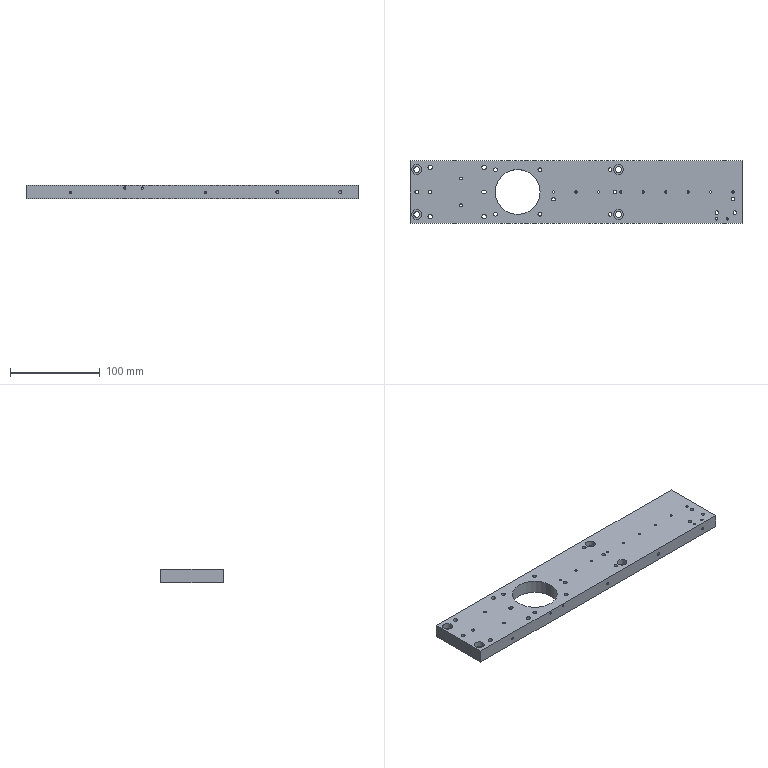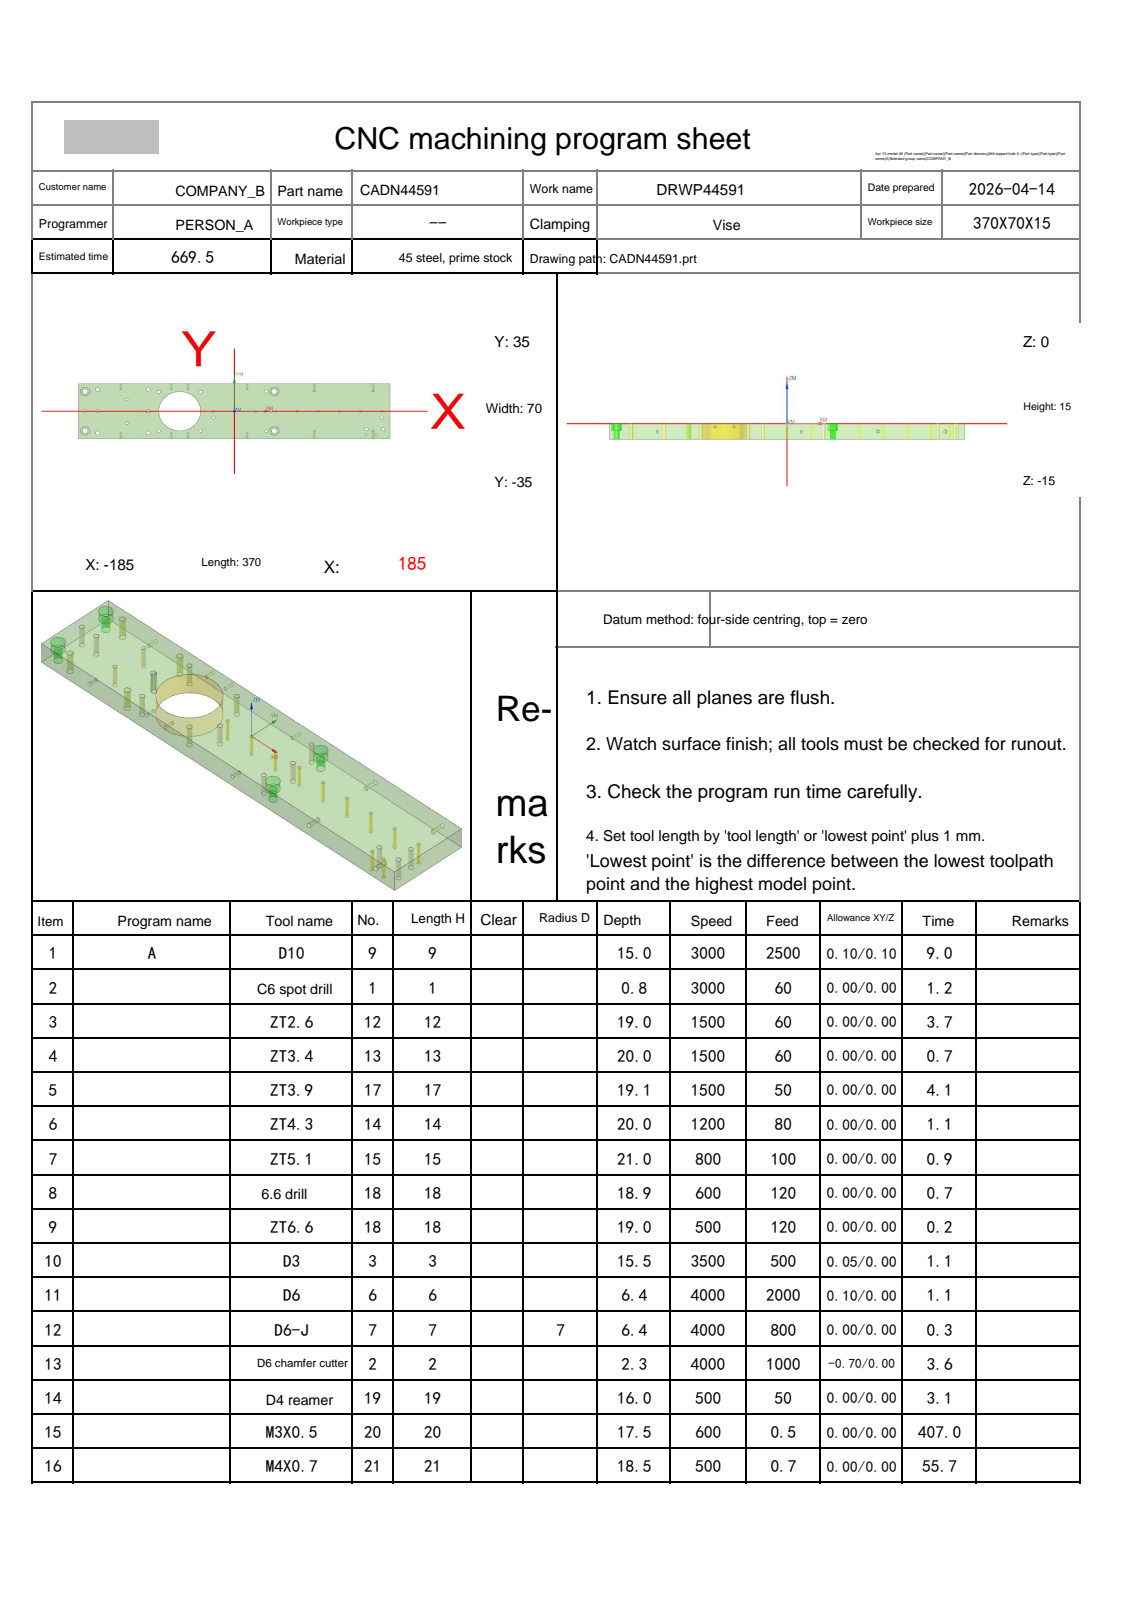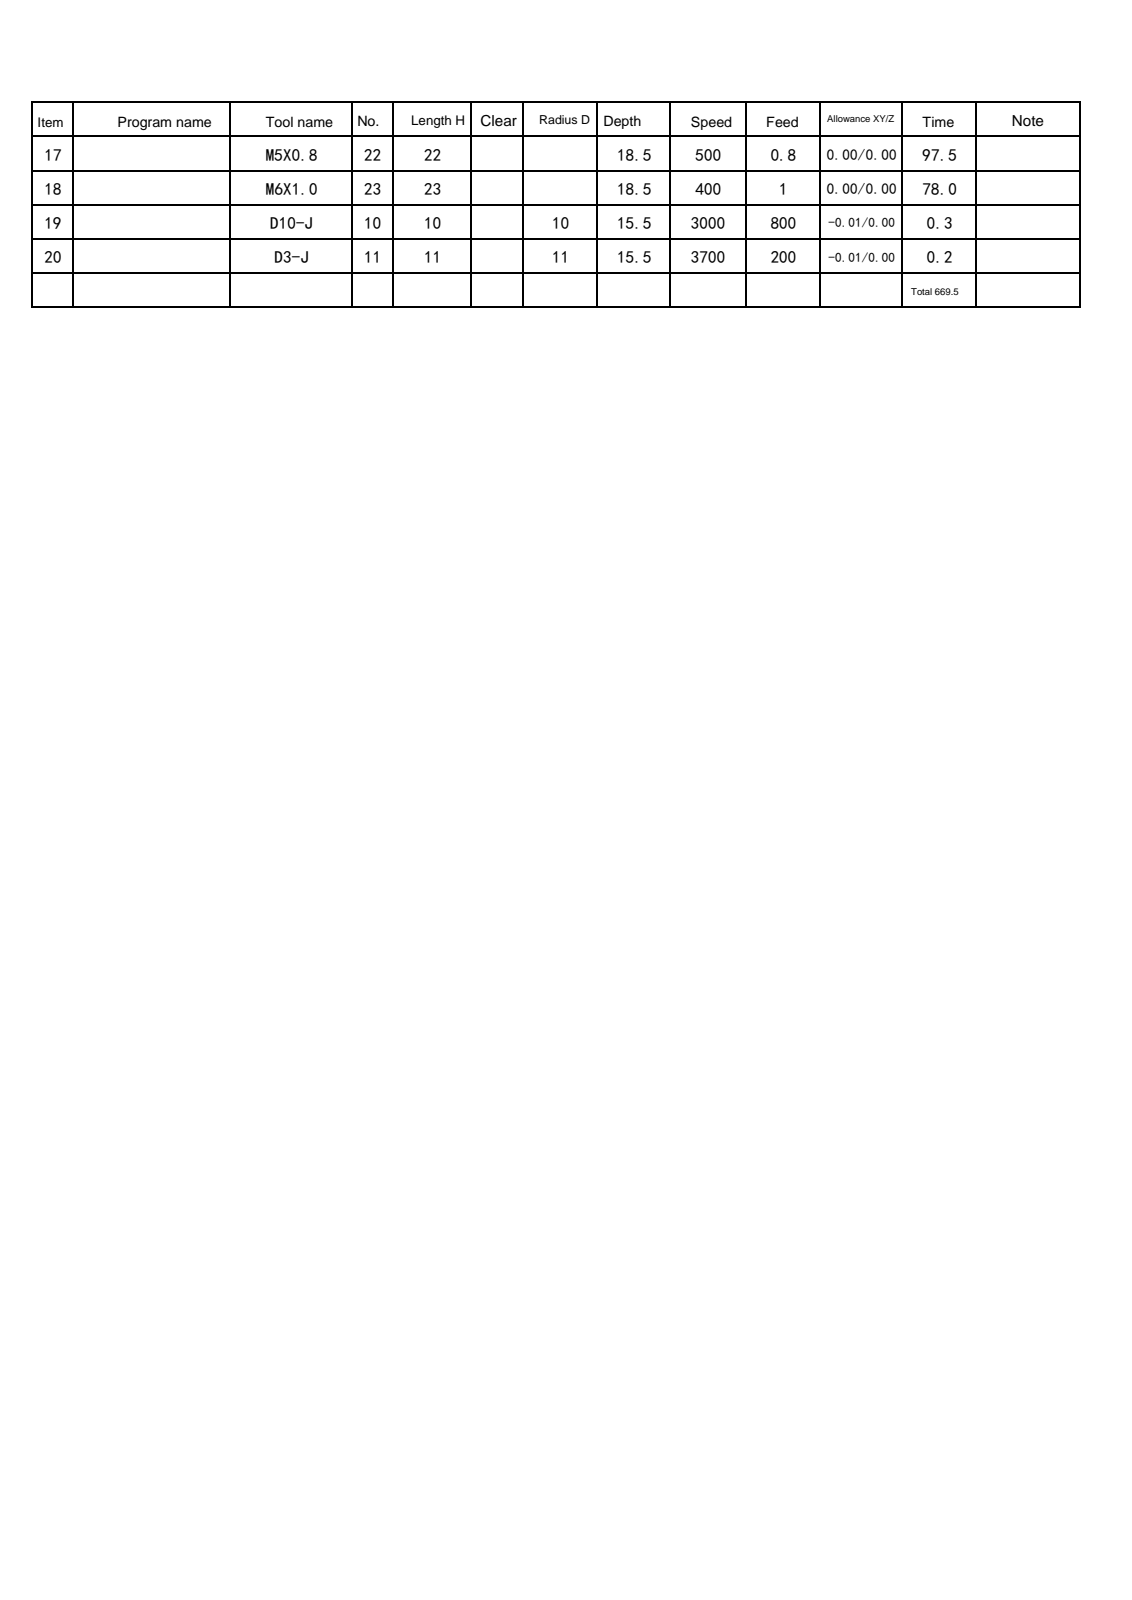NC program | NX | posted by the shop | part box 370 x 70 x 15 mm
Lines 2806 to 4500 of 4500, first 1279 of 1695 lines:
N2 T01 M06
(C6 spot drill  D=6. R=0. H=01 ce=0.00 di=0.10)
G00 G90 G54 X-65. Y0.0 M03 S3000
G43 H01 Z20.
M08
G98 G82 X-65. Y0.0 Z-.8 R1. F60.
X-103.
G80
G00 Z20.
G00 G90 X175. Y0.0 M03 S3000
Z20.
G98 G81 X175. Y0.0 Z-.8 R1. F60.
Y-8.
X177. Y-23.
X168.5 Y-30.
X156.5
X157. Y-23.
X150. Y0.0
X125.
X100.
X75.
X47.5 Y25.
X38.
X43.5 Y0.0
X50.
X47.5 Y-25.
X38.
X25. Y0.0
X0.0
X-25.
Y-8.
X-40.251 Y-24.749
Y24.749
X-89.749
X-102.5 Y27.5
X-128. Y15.
X-162.5 Y27.5
X-177.5 Y25.
Y0.0
X-162.5
X-177.5 Y-25.
X-162.5 Y-27.5
X-128. Y-15.
X-102.5 Y-27.5
X-89.749 Y-24.749
G80
G00 Z20.
G91 G28 Z0.0
M05
M09
G91 G28 Z0.0
M01
N3 T12 M06
(ZT2.6 D=2.6 DR_a=118 H=12)
G00 G90 G54 X156.5 Y-30. M03 S1500
G43 H12 Z20.
M08
G98 G83 X156.5 Y-30. Z-19. R1. F60. Q1.
X168.5
X175. Y0.0
X150.
X125.
X100.
X75.
X50.
X25.
X0.0
X-25.
G80
G00 Z20.
G91 G28 Z0.0
M05
M09
G91 G28 Z0.0
M01
N4 T13 M06
(ZT3.4 D=3.4 DR_a=118 H=13)
G00 G90 G54 X-128. Y-15. M03 S1500
G43 H13 Z20.
M08
G98 G83 X-128. Y-15. Z-20. R1. F60. Q1.
Y15.
G80
G00 Z20.
G91 G28 Z0.0
M05
M09
G91 G28 Z0.0
M01
N5 T17 M06
(ZT3.9 D=3.9 DR_a=120 H=17)
G00 G90 G54 X175. Y-8. M03 S1500
G43 H17 Z20.
M08
G98 G83 X175. Y-8. Z-19.126 R1. F50. Q1.
X177. Y-23.
X157.
X38. Y-25.
X43.5 Y0.0
X38. Y25.
X-25. Y-8.
X-162.5 Y0.0
X-177.5
X-103.
G80
G00 Z20.
G91 G28 Z0.0
M05
M09
G91 G28 Z0.0
M01
N6 T14 M06
(ZT4.3 D=4.3 DR_a=118 H=14)
G00 G90 G54 X-40.251 Y24.749 M03 S1200
G43 H14 Z20.
M08
G98 G83 X-40.251 Y24.749 Z-20. R1. F80. Q1.5
Y-24.749
X-89.749
Y24.749
G80
G00 Z20.
G91 G28 Z0.0
M05
M09
G91 G28 Z0.0
M01
N7 T15 M06
(ZT5.1 D=5.1 DR_a=118 H=15)
G00 G90 G54 X-162.5 Y27.5 M03 S800
G43 H15 Z20.
M08
G98 G83 X-162.5 Y27.5 Z-21. R1. F100. Q2.
Y-27.5
X-102.5
Y27.5
G80
G00 Z20.
G91 G28 Z0.0
M05
M09
G91 G28 Z0.0
M01
N8 T18 M06
(6.6 drill D=6.6 DR_a=120 H=18)
G00 G90 G54 X47.5 Y-25. M03 S600
G43 H18 Z20.
M08
G98 G83 X47.5 Y-25. Z-18.905 R1. F120. Q2.
Y25.
X-177.5
Y-25.
G80
G00 Z20.
G91 G28 Z0.0
M05
M09
G91 G28 Z0.0
M01
N9 T18 M06
(ZT6.6 D=6.6 DR_a=118 H=18)
G00 G90 G54 X-65. Y0.0 M03 S500
G43 H18 Z20.
M08
G98 G83 X-65. Y0.0 Z-18.983 R1. F120. Q2.
G80
G00 Z20.
G91 G28 Z0.0
M05
M09
G91 G28 Z0.0
M01
N10 T03 M06
(D3  D=3. R=0. H=03 ce=0.05 di=0.00)
G00 G90 G54 X-102.5 Y.45 M03 S3500
G43 H03 Z20.
M08
Z.5
G01 X-103. Z.485 F500.
G03 X-103.45 Y0.0 Z.463 I0.0 J-.45
X-103. Y-.45 Z.441 I.45 J0.0
G01 X-102. Z.41
G03 X-101.55 Y0.0 Z.388 I0.0 J.45
X-102. Y.45 Z.366 I-.45 J0.0
G01 X-103. Z.335
G03 X-103.45 Y0.0 Z.313 I0.0 J-.45
X-103. Y-.45 Z.291 I.45 J0.0
G01 X-102. Z.26
G03 X-101.55 Y0.0 Z.238 I0.0 J.45
X-102. Y.45 Z.216 I-.45 J0.0
G01 X-103. Z.185
G03 X-103.45 Y0.0 Z.164 I0.0 J-.45
X-103. Y-.45 Z.142 I.45 J0.0
G01 X-102. Z.111
G03 X-101.55 Y0.0 Z.089 I0.0 J.45
X-102. Y.45 Z.067 I-.45 J0.0
G01 X-103. Z.036
G03 X-103.45 Y0.0 Z.014 I0.0 J-.45
X-103. Y-.45 Z-.008 I.45 J0.0
G01 X-102. Z-.039
G03 X-101.55 Y0.0 Z-.061 I0.0 J.45
X-102. Y.45 Z-.083 I-.45 J0.0
G01 X-103. Z-.114
G03 X-103.45 Y0.0 Z-.136 I0.0 J-.45
X-103. Y-.45 Z-.157 I.45 J0.0
G01 X-102. Z-.188
G03 X-101.55 Y0.0 Z-.21 I0.0 J.45
X-102. Y.45 Z-.232 I-.45 J0.0
G01 X-103. Z-.263
G03 X-103.45 Y0.0 Z-.285 I0.0 J-.45
X-103. Y-.45 Z-.307 I.45 J0.0
G01 X-102. Z-.338
G03 X-101.55 Y0.0 Z-.36 I0.0 J.45
X-102. Y.45 Z-.382 I-.45 J0.0
G01 X-103. Z-.413
G03 X-103.45 Y0.0 Z-.435 I0.0 J-.45
X-103. Y-.45 Z-.456 I.45 J0.0
G01 X-102. Z-.487
G03 X-101.55 Y0.0 Z-.509 I0.0 J.45
X-102. Y.45 Z-.531 I-.45 J0.0
G01 X-103. Z-.562
G03 X-103.45 Y0.0 Z-.584 I0.0 J-.45
X-103. Y-.45 Z-.606 I.45 J0.0
G01 X-102. Z-.637
G03 X-101.55 Y0.0 Z-.659 I0.0 J.45
X-102. Y.45 Z-.681 I-.45 J0.0
G01 X-103. Z-.712
G03 X-103.45 Y0.0 Z-.734 I0.0 J-.45
X-103. Y-.45 Z-.756 I.45 J0.0
G01 X-102. Z-.787
G03 X-101.55 Y0.0 Z-.808 I0.0 J.45
X-102. Y.45 Z-.83 I-.45 J0.0
G01 X-103. Z-.861
G03 X-103.45 Y0.0 Z-.883 I0.0 J-.45
X-103. Y-.45 Z-.905 I.45 J0.0
G01 X-102. Z-.936
G03 X-101.55 Y0.0 Z-.958 I0.0 J.45
X-102. Y.45 Z-.98 I-.45 J0.0
G01 X-103. Z-1.011
G03 X-103.45 Y0.0 Z-1.033 I0.0 J-.45
X-103. Y-.45 Z-1.055 I.45 J0.0
G01 X-102. Z-1.086
G03 X-101.55 Y0.0 Z-1.107 I0.0 J.45
X-102. Y.45 Z-1.129 I-.45 J0.0
G01 X-103. Z-1.16
G03 X-103.45 Y0.0 Z-1.182 I0.0 J-.45
X-103. Y-.45 Z-1.204 I.45 J0.0
G01 X-102. Z-1.235
G03 X-101.55 Y0.0 Z-1.257 I0.0 J.45
X-102. Y.45 Z-1.279 I-.45 J0.0
G01 X-103. Z-1.31
G03 X-103.45 Y0.0 Z-1.332 I0.0 J-.45
X-103. Y-.45 Z-1.354 I.45 J0.0
G01 X-102. Z-1.385
G03 X-101.55 Y0.0 Z-1.407 I0.0 J.45
X-102. Y.45 Z-1.428 I-.45 J0.0
G01 X-103. Z-1.459
G03 X-103.45 Y0.0 Z-1.481 I0.0 J-.45
X-103. Y-.45 Z-1.503 I.45 J0.0
G01 X-102. Z-1.534
G03 X-101.55 Y0.0 Z-1.556 I0.0 J.45
X-102. Y.45 Z-1.578 I-.45 J0.0
G01 X-103. Z-1.609
G03 X-103.45 Y0.0 Z-1.631 I0.0 J-.45
X-103. Y-.45 Z-1.653 I.45 J0.0
G01 X-102. Z-1.684
G03 X-101.55 Y0.0 Z-1.706 I0.0 J.45
X-102. Y.45 Z-1.728 I-.45 J0.0
G01 X-103. Z-1.758
G03 X-103.45 Y0.0 Z-1.78 I0.0 J-.45
X-103. Y-.45 Z-1.802 I.45 J0.0
G01 X-102. Z-1.833
G03 X-101.55 Y0.0 Z-1.855 I0.0 J.45
X-102. Y.45 Z-1.877 I-.45 J0.0
G01 X-103. Z-1.908
G03 X-103.45 Y0.0 Z-1.93 I0.0 J-.45
X-103. Y-.45 Z-1.952 I.45 J0.0
G01 X-102. Z-1.983
G03 X-101.55 Y0.0 Z-2.005 I0.0 J.45
X-102. Y.45 Z-2.027 I-.45 J0.0
G01 X-103. Z-2.058
G03 X-103.45 Y0.0 Z-2.079 I0.0 J-.45
X-103. Y-.45 Z-2.101 I.45 J0.0
G01 X-102. Z-2.132
G03 X-101.55 Y0.0 Z-2.154 I0.0 J.45
X-102. Y.45 Z-2.176 I-.45 J0.0
G01 X-103. Z-2.207
G03 X-103.45 Y0.0 Z-2.229 I0.0 J-.45
X-103. Y-.45 Z-2.251 I.45 J0.0
G01 X-102. Z-2.282
G03 X-101.55 Y0.0 Z-2.304 I0.0 J.45
X-102. Y.45 Z-2.326 I-.45 J0.0
G01 X-103. Z-2.357
G03 X-103.45 Y0.0 Z-2.379 I0.0 J-.45
X-103. Y-.45 Z-2.4 I.45 J0.0
G01 X-102. Z-2.431
G03 X-101.55 Y0.0 Z-2.453 I0.0 J.45
X-102. Y.45 Z-2.475 I-.45 J0.0
G01 X-103. Z-2.506
G03 X-103.45 Y0.0 Z-2.528 I0.0 J-.45
X-103. Y-.45 Z-2.55 I.45 J0.0
G01 X-102. Z-2.581
G03 X-101.55 Y0.0 Z-2.603 I0.0 J.45
X-102. Y.45 Z-2.625 I-.45 J0.0
G01 X-103. Z-2.656
G03 X-103.45 Y0.0 Z-2.678 I0.0 J-.45
X-103. Y-.45 Z-2.699 I.45 J0.0
G01 X-102. Z-2.73
G03 X-101.55 Y0.0 Z-2.752 I0.0 J.45
X-102. Y.45 Z-2.774 I-.45 J0.0
G01 X-103. Z-2.805
G03 X-103.45 Y0.0 Z-2.827 I0.0 J-.45
X-103. Y-.45 Z-2.849 I.45 J0.0
G01 X-102. Z-2.88
G03 X-101.55 Y0.0 Z-2.902 I0.0 J.45
X-102. Y.45 Z-2.924 I-.45 J0.0
G01 X-103. Z-2.955
G03 X-103.45 Y0.0 Z-2.977 I0.0 J-.45
X-103. Y-.45 Z-2.999 I.45 J0.0
G01 X-102. Z-3.03
G03 X-101.55 Y0.0 Z-3.051 I0.0 J.45
X-102. Y.45 Z-3.073 I-.45 J0.0
G01 X-103. Z-3.104
G03 X-103.45 Y0.0 Z-3.126 I0.0 J-.45
X-103. Y-.45 Z-3.148 I.45 J0.0
G01 X-102. Z-3.179
G03 X-101.55 Y0.0 Z-3.201 I0.0 J.45
X-102. Y.45 Z-3.223 I-.45 J0.0
G01 X-103. Z-3.254
G03 X-103.45 Y0.0 Z-3.276 I0.0 J-.45
X-103. Y-.45 Z-3.298 I.45 J0.0
G01 X-102. Z-3.329
G03 X-101.55 Y0.0 Z-3.35 I0.0 J.45
X-102. Y.45 Z-3.372 I-.45 J0.0
G01 X-103. Z-3.403
G03 X-103.45 Y0.0 Z-3.425 I0.0 J-.45
X-103. Y-.45 Z-3.447 I.45 J0.0
G01 X-102. Z-3.478
G03 X-101.55 Y0.0 Z-3.5 I0.0 J.45
X-102. Y.45 Z-3.522 I-.45 J0.0
G01 X-103. Z-3.553
G03 X-103.45 Y0.0 Z-3.575 I0.0 J-.45
X-103. Y-.45 Z-3.597 I.45 J0.0
G01 X-102. Z-3.628
G03 X-101.55 Y0.0 Z-3.65 I0.0 J.45
X-102. Y.45 Z-3.671 I-.45 J0.0
G01 X-103. Z-3.702
G03 X-103.45 Y0.0 Z-3.724 I0.0 J-.45
X-103. Y-.45 Z-3.746 I.45 J0.0
G01 X-102. Z-3.777
G03 X-101.55 Y0.0 Z-3.799 I0.0 J.45
X-102. Y.45 Z-3.821 I-.45 J0.0
G01 X-103. Z-3.852
G03 X-103.45 Y0.0 Z-3.874 I0.0 J-.45
X-103. Y-.45 Z-3.896 I.45 J0.0
G01 X-102. Z-3.927
G03 X-101.55 Y0.0 Z-3.949 I0.0 J.45
X-102. Y.45 Z-3.97 I-.45 J0.0
G01 X-103. Z-4.001
G03 X-103.45 Y0.0 Z-4.023 I0.0 J-.45
X-103. Y-.45 Z-4.045 I.45 J0.0
G01 X-102. Z-4.076
G03 X-101.55 Y0.0 Z-4.098 I0.0 J.45
X-102. Y.45 Z-4.12 I-.45 J0.0
G01 X-103. Z-4.151
G03 X-103.45 Y0.0 Z-4.173 I0.0 J-.45
X-103. Y-.45 Z-4.195 I.45 J0.0
G01 X-102. Z-4.226
G03 X-101.55 Y0.0 Z-4.248 I0.0 J.45
X-102. Y.45 Z-4.27 I-.45 J0.0
G01 X-103. Z-4.301
G03 X-103.45 Y0.0 Z-4.322 I0.0 J-.45
X-103. Y-.45 Z-4.344 I.45 J0.0
G01 X-102. Z-4.375
G03 X-101.55 Y0.0 Z-4.397 I0.0 J.45
X-102. Y.45 Z-4.419 I-.45 J0.0
G01 X-103. Z-4.45
G03 X-103.45 Y0.0 Z-4.472 I0.0 J-.45
X-103. Y-.45 Z-4.494 I.45 J0.0
G01 X-102. Z-4.525
G03 X-101.55 Y0.0 Z-4.547 I0.0 J.45
X-102. Y.45 Z-4.569 I-.45 J0.0
G01 X-103. Z-4.6
G03 X-103.45 Y0.0 Z-4.621 I0.0 J-.45
X-103. Y-.45 Z-4.643 I.45 J0.0
G01 X-102. Z-4.674
G03 X-101.55 Y0.0 Z-4.696 I0.0 J.45
X-102. Y.45 Z-4.718 I-.45 J0.0
G01 X-103. Z-4.749
G03 X-103.45 Y0.0 Z-4.771 I0.0 J-.45
X-103. Y-.45 Z-4.793 I.45 J0.0
G01 X-102. Z-4.824
G03 X-101.55 Y0.0 Z-4.846 I0.0 J.45
X-102. Y.45 Z-4.868 I-.45 J0.0
G01 X-103. Z-4.899
G03 X-103.45 Y0.0 Z-4.921 I0.0 J-.45
X-103. Y-.45 Z-4.942 I.45 J0.0
G01 X-102. Z-4.973
G03 X-101.55 Y0.0 Z-4.995 I0.0 J.45
X-102. Y.45 Z-5.017 I-.45 J0.0
G01 X-103. Z-5.048
G03 X-103.45 Y0.0 Z-5.07 I0.0 J-.45
X-103. Y-.45 Z-5.092 I.45 J0.0
G01 X-102. Z-5.123
G03 X-101.55 Y0.0 Z-5.145 I0.0 J.45
X-102. Y.45 Z-5.167 I-.45 J0.0
G01 X-103. Z-5.198
G03 X-103.45 Y0.0 Z-5.22 I0.0 J-.45
X-103. Y-.45 Z-5.242 I.45 J0.0
G01 X-102. Z-5.272
G03 X-101.55 Y0.0 Z-5.294 I0.0 J.45
X-102. Y.45 Z-5.316 I-.45 J0.0
G01 X-103. Z-5.347
G03 X-103.45 Y0.0 Z-5.369 I0.0 J-.45
X-103. Y-.45 Z-5.391 I.45 J0.0
G01 X-102. Z-5.422
G03 X-101.55 Y0.0 Z-5.444 I0.0 J.45
X-102. Y.45 Z-5.466 I-.45 J0.0
G01 X-103. Z-5.497
G03 X-103.45 Y0.0 Z-5.519 I0.0 J-.45
X-103. Y-.45 Z-5.541 I.45 J0.0
G01 X-102. Z-5.572
G03 X-101.55 Y0.0 Z-5.593 I0.0 J.45
X-102. Y.45 Z-5.615 I-.45 J0.0
G01 X-103. Z-5.646
G03 X-103.45 Y0.0 Z-5.668 I0.0 J-.45
X-103. Y-.45 Z-5.69 I.45 J0.0
G01 X-102. Z-5.721
G03 X-101.55 Y0.0 Z-5.743 I0.0 J.45
X-102. Y.45 Z-5.765 I-.45 J0.0
G01 X-103. Z-5.796
G03 X-103.45 Y0.0 Z-5.818 I0.0 J-.45
X-103. Y-.45 Z-5.84 I.45 J0.0
G01 X-102. Z-5.871
G03 X-101.55 Y0.0 Z-5.893 I0.0 J.45
X-102. Y.45 Z-5.914 I-.45 J0.0
G01 X-103. Z-5.945
G03 X-103.45 Y0.0 Z-5.967 I0.0 J-.45
X-103. Y-.45 Z-5.989 I.45 J0.0
G01 X-102. Z-6.02
G03 X-101.55 Y0.0 Z-6.042 I0.0 J.45
X-102. Y.45 Z-6.064 I-.45 J0.0
G01 X-103. Z-6.095
G03 X-103.45 Y0.0 Z-6.117 I0.0 J-.45
X-103. Y-.45 Z-6.139 I.45 J0.0
G01 X-102. Z-6.17
G03 X-101.55 Y0.0 Z-6.192 I0.0 J.45
X-102. Y.45 Z-6.213 I-.45 J0.0
G01 X-103. Z-6.244
G03 X-103.45 Y0.0 Z-6.266 I0.0 J-.45
X-103. Y-.45 Z-6.288 I.45 J0.0
G01 X-102. Z-6.319
G03 X-101.55 Y0.0 Z-6.341 I0.0 J.45
X-102. Y.45 Z-6.363 I-.45 J0.0
G01 X-103. Z-6.394
G03 X-103.45 Y0.0 Z-6.416 I0.0 J-.45
X-103. Y-.45 Z-6.438 I.45 J0.0
G01 X-102. Z-6.469
G03 X-101.55 Y0.0 Z-6.491 I0.0 J.45
X-102. Y.45 Z-6.513 I-.45 J0.0
G01 X-103. Z-6.544
G03 X-103.45 Y0.0 Z-6.565 I0.0 J-.45
X-103. Y-.45 Z-6.587 I.45 J0.0
G01 X-102. Z-6.618
G03 X-101.55 Y0.0 Z-6.64 I0.0 J.45
X-102. Y.45 Z-6.662 I-.45 J0.0
G01 X-103. Z-6.693
G03 X-103.45 Y0.0 Z-6.715 I0.0 J-.45
X-103. Y-.45 Z-6.737 I.45 J0.0
G01 X-102. Z-6.768
G03 X-101.55 Y0.0 Z-6.79 I0.0 J.45
X-102. Y.45 Z-6.812 I-.45 J0.0
G01 X-103. Z-6.843
G03 X-103.45 Y0.0 Z-6.864 I0.0 J-.45
X-103. Y-.45 Z-6.886 I.45 J0.0
G01 X-102. Z-6.917
G03 X-101.55 Y0.0 Z-6.939 I0.0 J.45
X-102. Y.45 Z-6.961 I-.45 J0.0
G01 X-103. Z-6.992
G03 X-103.45 Y0.0 Z-7.014 I0.0 J-.45
X-103. Y-.45 Z-7.036 I.45 J0.0
G01 X-102. Z-7.067
G03 X-101.55 Y0.0 Z-7.089 I0.0 J.45
X-102. Y.45 Z-7.111 I-.45 J0.0
G01 X-103. Z-7.142
G03 X-103.45 Y0.0 Z-7.164 I0.0 J-.45
X-103. Y-.45 Z-7.185 I.45 J0.0
G01 X-102. Z-7.216
G03 X-101.55 Y0.0 Z-7.238 I0.0 J.45
X-102. Y.45 Z-7.26 I-.45 J0.0
G01 X-103. Z-7.291
G03 X-103.45 Y0.0 Z-7.313 I0.0 J-.45
X-103. Y-.45 Z-7.335 I.45 J0.0
G01 X-102. Z-7.366
G03 X-101.55 Y0.0 Z-7.388 I0.0 J.45
X-102. Y.45 Z-7.41 I-.45 J0.0
G01 X-103. Z-7.441
G03 X-103.45 Y0.0 Z-7.463 I0.0 J-.45
X-103. Y-.45 Z-7.485 I.45 J0.0
G01 X-102. Z-7.515
G03 X-101.55 Y0.0 Z-7.537 I0.0 J.45
X-102. Y.45 Z-7.559 I-.45 J0.0
G01 X-103. Z-7.59
G03 X-103.45 Y0.0 Z-7.612 I0.0 J-.45
X-103. Y-.45 Z-7.634 I.45 J0.0
G01 X-102. Z-7.665
G03 X-101.55 Y0.0 Z-7.687 I0.0 J.45
X-102. Y.45 Z-7.709 I-.45 J0.0
G01 X-103. Z-7.74
G03 X-103.45 Y0.0 Z-7.762 I0.0 J-.45
X-103. Y-.45 Z-7.784 I.45 J0.0
G01 X-102. Z-7.815
G03 X-101.55 Y0.0 Z-7.836 I0.0 J.45
X-102. Y.45 Z-7.858 I-.45 J0.0
G01 X-103. Z-7.889
G03 X-103.45 Y0.0 Z-7.911 I0.0 J-.45
X-103. Y-.45 Z-7.933 I.45 J0.0
G01 X-102. Z-7.964
G03 X-101.55 Y0.0 Z-7.986 I0.0 J.45
X-102. Y.45 Z-8.008 I-.45 J0.0
G01 X-103. Z-8.039
G03 X-103.45 Y0.0 Z-8.061 I0.0 J-.45
X-103. Y-.45 Z-8.083 I.45 J0.0
G01 X-102. Z-8.114
G03 X-101.55 Y0.0 Z-8.136 I0.0 J.45
X-102. Y.45 Z-8.157 I-.45 J0.0
G01 X-103. Z-8.188
G03 X-103.45 Y0.0 Z-8.21 I0.0 J-.45
X-103. Y-.45 Z-8.232 I.45 J0.0
G01 X-102. Z-8.263
G03 X-101.55 Y0.0 Z-8.285 I0.0 J.45
X-102. Y.45 Z-8.307 I-.45 J0.0
G01 X-103. Z-8.338
G03 X-103.45 Y0.0 Z-8.36 I0.0 J-.45
X-103. Y-.45 Z-8.382 I.45 J0.0
G01 X-102. Z-8.413
G03 X-101.55 Y0.0 Z-8.435 I0.0 J.45
X-102. Y.45 Z-8.456 I-.45 J0.0
G01 X-103. Z-8.487
G03 X-103.45 Y0.0 Z-8.509 I0.0 J-.45
X-103. Y-.45 Z-8.531 I.45 J0.0
G01 X-102. Z-8.562
G03 X-101.55 Y0.0 Z-8.584 I0.0 J.45
X-102. Y.45 Z-8.606 I-.45 J0.0
G01 X-103. Z-8.637
G03 X-103.45 Y0.0 Z-8.659 I0.0 J-.45
X-103. Y-.45 Z-8.681 I.45 J0.0
G01 X-102. Z-8.712
G03 X-101.55 Y0.0 Z-8.734 I0.0 J.45
X-102. Y.45 Z-8.756 I-.45 J0.0
G01 X-103. Z-8.787
G03 X-103.45 Y0.0 Z-8.808 I0.0 J-.45
X-103. Y-.45 Z-8.83 I.45 J0.0
G01 X-102. Z-8.861
G03 X-101.55 Y0.0 Z-8.883 I0.0 J.45
X-102. Y.45 Z-8.905 I-.45 J0.0
G01 X-103. Z-8.936
G03 X-103.45 Y0.0 Z-8.958 I0.0 J-.45
X-103. Y-.45 Z-8.98 I.45 J0.0
G01 X-102. Z-9.011
G03 X-101.55 Y0.0 Z-9.033 I0.0 J.45
X-102. Y.45 Z-9.055 I-.45 J0.0
G01 X-103. Z-9.086
G03 X-103.45 Y0.0 Z-9.107 I0.0 J-.45
X-103. Y-.45 Z-9.129 I.45 J0.0
G01 X-102. Z-9.16
G03 X-101.55 Y0.0 Z-9.182 I0.0 J.45
X-102. Y.45 Z-9.204 I-.45 J0.0
G01 X-103. Z-9.235
G03 X-103.45 Y0.0 Z-9.257 I0.0 J-.45
X-103. Y-.45 Z-9.279 I.45 J0.0
G01 X-102. Z-9.31
G03 X-101.55 Y0.0 Z-9.332 I0.0 J.45
X-102. Y.45 Z-9.354 I-.45 J0.0
G01 X-103. Z-9.385
G03 X-103.45 Y0.0 Z-9.407 I0.0 J-.45
X-103. Y-.45 Z-9.428 I.45 J0.0
G01 X-102. Z-9.459
G03 X-101.55 Y0.0 Z-9.481 I0.0 J.45
X-102. Y.45 Z-9.503 I-.45 J0.0
G01 X-103. Z-9.534
G03 X-103.45 Y0.0 Z-9.556 I0.0 J-.45
X-103. Y-.45 Z-9.578 I.45 J0.0
G01 X-102. Z-9.609
G03 X-101.55 Y0.0 Z-9.631 I0.0 J.45
X-102. Y.45 Z-9.653 I-.45 J0.0
G01 X-103. Z-9.684
G03 X-103.45 Y0.0 Z-9.706 I0.0 J-.45
X-103. Y-.45 Z-9.728 I.45 J0.0
G01 X-102. Z-9.758
G03 X-101.55 Y0.0 Z-9.78 I0.0 J.45
X-102. Y.45 Z-9.802 I-.45 J0.0
G01 X-103. Z-9.833
G03 X-103.45 Y0.0 Z-9.855 I0.0 J-.45
X-103. Y-.45 Z-9.877 I.45 J0.0
G01 X-102. Z-9.908
G03 X-101.55 Y0.0 Z-9.93 I0.0 J.45
X-102. Y.45 Z-9.952 I-.45 J0.0
G01 X-103. Z-9.983
G03 X-103.45 Y0.0 Z-10.005 I0.0 J-.45
X-103. Y-.45 Z-10.027 I.45 J0.0
G01 X-102. Z-10.058
G03 X-101.55 Y0.0 Z-10.079 I0.0 J.45
X-102. Y.45 Z-10.101 I-.45 J0.0
G01 X-103. Z-10.132
G03 X-103.45 Y0.0 Z-10.154 I0.0 J-.45
X-103. Y-.45 Z-10.176 I.45 J0.0
G01 X-102. Z-10.207
G03 X-101.55 Y0.0 Z-10.229 I0.0 J.45
X-102. Y.45 Z-10.251 I-.45 J0.0
G01 X-103. Z-10.282
G03 X-103.45 Y0.0 Z-10.304 I0.0 J-.45
X-103. Y-.45 Z-10.326 I.45 J0.0
G01 X-102. Z-10.357
G03 X-101.55 Y0.0 Z-10.379 I0.0 J.45
X-102. Y.45 Z-10.4 I-.45 J0.0
G01 X-103. Z-10.431
G03 X-103.45 Y0.0 Z-10.453 I0.0 J-.45
X-103. Y-.45 Z-10.475 I.45 J0.0
G01 X-102. Z-10.506
G03 X-101.55 Y0.0 Z-10.528 I0.0 J.45
X-102. Y.45 Z-10.55 I-.45 J0.0
G01 X-103. Z-10.581
G03 X-103.45 Y0.0 Z-10.603 I0.0 J-.45
X-103. Y-.45 Z-10.625 I.45 J0.0
G01 X-102. Z-10.656
G03 X-101.55 Y0.0 Z-10.678 I0.0 J.45
X-102. Y.45 Z-10.699 I-.45 J0.0
G01 X-103. Z-10.73
G03 X-103.45 Y0.0 Z-10.752 I0.0 J-.45
X-103. Y-.45 Z-10.774 I.45 J0.0
G01 X-102. Z-10.805
G03 X-101.55 Y0.0 Z-10.827 I0.0 J.45
X-102. Y.45 Z-10.849 I-.45 J0.0
G01 X-103. Z-10.88
G03 X-103.45 Y0.0 Z-10.902 I0.0 J-.45
X-103. Y-.45 Z-10.924 I.45 J0.0
G01 X-102. Z-10.955
G03 X-101.55 Y0.0 Z-10.977 I0.0 J.45
X-102. Y.45 Z-10.999 I-.45 J0.0
G01 X-103. Z-11.03
G03 X-103.45 Y0.0 Z-11.051 I0.0 J-.45
X-103. Y-.45 Z-11.073 I.45 J0.0
G01 X-102. Z-11.104
G03 X-101.55 Y0.0 Z-11.126 I0.0 J.45
X-102. Y.45 Z-11.148 I-.45 J0.0
G01 X-103. Z-11.179
G03 X-103.45 Y0.0 Z-11.201 I0.0 J-.45
X-103. Y-.45 Z-11.223 I.45 J0.0
G01 X-102. Z-11.254
G03 X-101.55 Y0.0 Z-11.276 I0.0 J.45
X-102. Y.45 Z-11.298 I-.45 J0.0
G01 X-103. Z-11.329
G03 X-103.45 Y0.0 Z-11.35 I0.0 J-.45
X-103. Y-.45 Z-11.372 I.45 J0.0
G01 X-102. Z-11.403
G03 X-101.55 Y0.0 Z-11.425 I0.0 J.45
X-102. Y.45 Z-11.447 I-.45 J0.0
G01 X-103. Z-11.478
G03 X-103.45 Y0.0 Z-11.5 I0.0 J-.45
X-103. Y-.45 Z-11.522 I.45 J0.0
G01 X-102. Z-11.553
G03 X-101.55 Y0.0 Z-11.575 I0.0 J.45
X-102. Y.45 Z-11.597 I-.45 J0.0
G01 X-103. Z-11.628
G03 X-103.45 Y0.0 Z-11.65 I0.0 J-.45
X-103. Y-.45 Z-11.671 I.45 J0.0
G01 X-102. Z-11.702
G03 X-101.55 Y0.0 Z-11.724 I0.0 J.45
X-102. Y.45 Z-11.746 I-.45 J0.0
G01 X-103. Z-11.777
G03 X-103.45 Y0.0 Z-11.799 I0.0 J-.45
X-103. Y-.45 Z-11.821 I.45 J0.0
G01 X-102. Z-11.852
G03 X-101.55 Y0.0 Z-11.874 I0.0 J.45
X-102. Y.45 Z-11.896 I-.45 J0.0
G01 X-103. Z-11.927
G03 X-103.45 Y0.0 Z-11.949 I0.0 J-.45
X-103. Y-.45 Z-11.97 I.45 J0.0
G01 X-102. Z-12.001
G03 X-101.55 Y0.0 Z-12.023 I0.0 J.45
X-102. Y.45 Z-12.045 I-.45 J0.0
G01 X-103. Z-12.076
G03 X-103.45 Y0.0 Z-12.098 I0.0 J-.45
X-103. Y-.45 Z-12.12 I.45 J0.0
G01 X-102. Z-12.151
G03 X-101.55 Y0.0 Z-12.173 I0.0 J.45
X-102. Y.45 Z-12.195 I-.45 J0.0
G01 X-103. Z-12.226
G03 X-103.45 Y0.0 Z-12.248 I0.0 J-.45
X-103. Y-.45 Z-12.27 I.45 J0.0
G01 X-102. Z-12.301
G03 X-101.55 Y0.0 Z-12.322 I0.0 J.45
X-102. Y.45 Z-12.344 I-.45 J0.0
G01 X-103. Z-12.375
G03 X-103.45 Y0.0 Z-12.397 I0.0 J-.45
X-103. Y-.45 Z-12.419 I.45 J0.0
G01 X-102. Z-12.45
G03 X-101.55 Y0.0 Z-12.472 I0.0 J.45
X-102. Y.45 Z-12.494 I-.45 J0.0
G01 X-103. Z-12.525
G03 X-103.45 Y0.0 Z-12.547 I0.0 J-.45
X-103. Y-.45 Z-12.569 I.45 J0.0
G01 X-102. Z-12.6
G03 X-101.55 Y0.0 Z-12.621 I0.0 J.45
X-102. Y.45 Z-12.643 I-.45 J0.0
G01 X-103. Z-12.674
G03 X-103.45 Y0.0 Z-12.696 I0.0 J-.45
X-103. Y-.45 Z-12.718 I.45 J0.0
G01 X-102. Z-12.749
G03 X-101.55 Y0.0 Z-12.771 I0.0 J.45
X-102. Y.45 Z-12.793 I-.45 J0.0
G01 X-103. Z-12.824
G03 X-103.45 Y0.0 Z-12.846 I0.0 J-.45
X-103. Y-.45 Z-12.868 I.45 J0.0
G01 X-102. Z-12.899
G03 X-101.55 Y0.0 Z-12.921 I0.0 J.45
X-102. Y.45 Z-12.942 I-.45 J0.0
G01 X-103. Z-12.973
G03 X-103.45 Y0.0 Z-12.995 I0.0 J-.45
X-103. Y-.45 Z-13.017 I.45 J0.0
G01 X-102. Z-13.048
G03 X-101.55 Y0.0 Z-13.07 I0.0 J.45
X-102. Y.45 Z-13.092 I-.45 J0.0
G01 X-103. Z-13.123
G03 X-103.45 Y0.0 Z-13.145 I0.0 J-.45
X-103. Y-.45 Z-13.167 I.45 J0.0
G01 X-102. Z-13.198
G03 X-101.55 Y0.0 Z-13.22 I0.0 J.45
X-102. Y.45 Z-13.242 I-.45 J0.0
G01 X-103. Z-13.272
G03 X-103.45 Y0.0 Z-13.294 I0.0 J-.45
X-103. Y-.45 Z-13.316 I.45 J0.0
G01 X-102. Z-13.347
G03 X-101.55 Y0.0 Z-13.369 I0.0 J.45
X-102. Y.45 Z-13.391 I-.45 J0.0
G01 X-103. Z-13.422
G03 X-103.45 Y0.0 Z-13.444 I0.0 J-.45
X-103. Y-.45 Z-13.466 I.45 J0.0
G01 X-102. Z-13.497
G03 X-101.55 Y0.0 Z-13.519 I0.0 J.45
X-102. Y.45 Z-13.541 I-.45 J0.0
G01 X-103. Z-13.572
G03 X-103.45 Y0.0 Z-13.593 I0.0 J-.45
X-103. Y-.45 Z-13.615 I.45 J0.0
G01 X-102. Z-13.646
G03 X-101.55 Y0.0 Z-13.668 I0.0 J.45
X-102. Y.45 Z-13.69 I-.45 J0.0
G01 X-103. Z-13.721
G03 X-103.45 Y0.0 Z-13.743 I0.0 J-.45
X-103. Y-.45 Z-13.765 I.45 J0.0
G01 X-102. Z-13.796
G03 X-101.55 Y0.0 Z-13.818 I0.0 J.45
X-102. Y.45 Z-13.84 I-.45 J0.0
G01 X-103. Z-13.871
G03 X-103.45 Y0.0 Z-13.893 I0.0 J-.45
X-103. Y-.45 Z-13.914 I.45 J0.0
G01 X-102. Z-13.945
G03 X-101.55 Y0.0 Z-13.967 I0.0 J.45
X-102. Y.45 Z-13.989 I-.45 J0.0
G01 X-103. Z-14.02
G03 X-103.45 Y0.0 Z-14.042 I0.0 J-.45
X-103. Y-.45 Z-14.064 I.45 J0.0
G01 X-102. Z-14.095
G03 X-101.55 Y0.0 Z-14.117 I0.0 J.45
X-102. Y.45 Z-14.139 I-.45 J0.0
G01 X-103. Z-14.17
G03 X-103.45 Y0.0 Z-14.192 I0.0 J-.45
X-103. Y-.45 Z-14.213 I.45 J0.0
G01 X-102. Z-14.244
G03 X-101.55 Y0.0 Z-14.266 I0.0 J.45
X-102. Y.45 Z-14.288 I-.45 J0.0
G01 X-103. Z-14.319
G03 X-103.45 Y0.0 Z-14.341 I0.0 J-.45
X-103. Y-.45 Z-14.363 I.45 J0.0
G01 X-102. Z-14.394
G03 X-101.55 Y0.0 Z-14.416 I0.0 J.45
X-102. Y.45 Z-14.438 I-.45 J0.0
G01 X-103. Z-14.469
G03 X-103.45 Y0.0 Z-14.491 I0.0 J-.45
X-103. Y-.45 Z-14.513 I.45 J0.0
G01 X-102. Z-14.544
G03 X-101.55 Y0.0 Z-14.565 I0.0 J.45
X-102. Y.45 Z-14.587 I-.45 J0.0
G01 X-103. Z-14.618
G03 X-103.45 Y0.0 Z-14.64 I0.0 J-.45
X-103. Y-.45 Z-14.662 I.45 J0.0
G01 X-102. Z-14.693
G03 X-101.55 Y0.0 Z-14.715 I0.0 J.45
X-102. Y.45 Z-14.737 I-.45 J0.0
G01 X-103. Z-14.768
G03 X-103.45 Y0.0 Z-14.79 I0.0 J-.45
X-103. Y-.45 Z-14.812 I.45 J0.0
G01 X-102. Z-14.843
G03 X-101.55 Y0.0 Z-14.864 I0.0 J.45
X-102. Y.45 Z-14.886 I-.45 J0.0
G01 X-103. Z-14.917
G03 X-103.45 Y0.0 Z-14.939 I0.0 J-.45
X-103. Y-.45 Z-14.961 I.45 J0.0
G01 X-102. Z-14.992
G03 X-101.55 Y0.0 Z-15.014 I0.0 J.45
X-102. Y.45 Z-15.036 I-.45 J0.0
G01 X-103. Z-15.067
G03 X-103.45 Y0.0 Z-15.089 I0.0 J-.45
X-103. Y-.45 Z-15.111 I.45 J0.0
G01 X-102. Z-15.142
G03 X-101.55 Y0.0 Z-15.164 I0.0 J.45
X-102. Y.45 Z-15.185 I-.45 J0.0
G01 X-103. Z-15.216
G03 X-103.45 Y0.0 Z-15.238 I0.0 J-.45
X-103. Y-.45 Z-15.26 I.45 J0.0
G01 X-102. Z-15.291
G03 X-101.55 Y0.0 Z-15.313 I0.0 J.45
X-102. Y.45 Z-15.335 I-.45 J0.0
G01 X-103. Z-15.366
G03 X-103.45 Y0.0 Z-15.388 I0.0 J-.45
X-103. Y-.45 Z-15.41 I.45 J0.0
G01 X-102. Z-15.441
G03 X-101.55 Y0.0 Z-15.463 I0.0 J.45
X-102. Y.45 Z-15.485 I-.45 J0.0
G01 X-102.5 Z-15.5
X-103.
G03 X-103.45 Y0.0 I0.0 J-.45
X-103. Y-.45 I.45 J0.0
G01 X-102.
G03 X-101.55 Y0.0 I0.0 J.45
X-102. Y.45 I-.45 J0.0
G01 X-102.5
X-103.
Z-14.5
G00 Z20.
G91 G28 Z0.0
M05
M09
G91 G28 Z0.0
M01
N11 T06 M06
(D6  D=6. R=0. H=06 ce=0.10 di=0.00)
G00 G90 G54 X47.5 Y-25. M03 S4000
G43 H06 Z20.
M08
Z.5
G03 X48.7 Y-26.2 I1.2 J0.0 F2000.
X49.9 Y-25. I0.0 J1.2
X49.9 Y-25. Z.3 I-2.4 J0.0
X49.9 Y-25. Z.1 I-2.4 J0.0
X49.9 Y-25. Z-.1 I-2.4 J0.0
X49.9 Y-25. Z-.3 I-2.4 J0.0
X49.9 Y-25. Z-.5 I-2.4 J0.0
X49.9 Y-25. Z-.7 I-2.4 J0.0
X49.9 Y-25. Z-.9 I-2.4 J0.0
X49.9 Y-25. Z-1.1 I-2.4 J0.0
X49.9 Y-25. Z-1.3 I-2.4 J0.0
X49.9 Y-25. Z-1.5 I-2.4 J0.0
X49.9 Y-25. Z-1.7 I-2.4 J0.0
X49.9 Y-25. Z-1.9 I-2.4 J0.0
X49.9 Y-25. Z-2.1 I-2.4 J0.0
X49.9 Y-25. Z-2.3 I-2.4 J0.0
X49.9 Y-25. Z-2.5 I-2.4 J0.0
X49.9 Y-25. Z-2.7 I-2.4 J0.0
X49.9 Y-25. Z-2.9 I-2.4 J0.0
X49.9 Y-25. Z-3.1 I-2.4 J0.0
X49.9 Y-25. Z-3.3 I-2.4 J0.0
X49.9 Y-25. Z-3.5 I-2.4 J0.0
X49.9 Y-25. Z-3.7 I-2.4 J0.0
X49.9 Y-25. Z-3.9 I-2.4 J0.0
X49.9 Y-25. Z-4.1 I-2.4 J0.0
X49.9 Y-25. Z-4.3 I-2.4 J0.0
X49.9 Y-25. Z-4.5 I-2.4 J0.0
X49.9 Y-25. Z-4.7 I-2.4 J0.0
X49.9 Y-25. Z-4.9 I-2.4 J0.0
X49.9 Y-25. Z-5.1 I-2.4 J0.0
X49.9 Y-25. Z-5.3 I-2.4 J0.0
X49.9 Y-25. Z-5.5 I-2.4 J0.0
X49.9 Y-25. Z-5.7 I-2.4 J0.0
X49.9 Y-25. Z-5.9 I-2.4 J0.0
X49.9 Y-25. Z-6.1 I-2.4 J0.0
X49.9 Y-25. Z-6.3 I-2.4 J0.0
X45.1 Y-25. Z-6.4 I-2.4 J0.0
X47.5 Y-27.4 I2.4 J0.0
X49.9 Y-25. I0.0 J2.4
X47.5 Y-22.6 I-2.4 J0.0
X45.1 Y-25. I0.0 J-2.4
X46.3 Y-26.2 I1.2 J0.0
X47.5 Y-25. I0.0 J1.2
G00 Z20.
Y25.
Z.5
G03 X48.7 Y23.8 I1.2 J0.0
X49.9 Y25. I0.0 J1.2
X49.9 Y25. Z.3 I-2.4 J0.0
X49.9 Y25. Z.1 I-2.4 J0.0
X49.9 Y25. Z-.1 I-2.4 J0.0
X49.9 Y25. Z-.3 I-2.4 J0.0
X49.9 Y25. Z-.5 I-2.4 J0.0
X49.9 Y25. Z-.7 I-2.4 J0.0
X49.9 Y25. Z-.9 I-2.4 J0.0
X49.9 Y25. Z-1.1 I-2.4 J0.0
X49.9 Y25. Z-1.3 I-2.4 J0.0
X49.9 Y25. Z-1.5 I-2.4 J0.0
X49.9 Y25. Z-1.7 I-2.4 J0.0
X49.9 Y25. Z-1.9 I-2.4 J0.0
X49.9 Y25. Z-2.1 I-2.4 J0.0
X49.9 Y25. Z-2.3 I-2.4 J0.0
X49.9 Y25. Z-2.5 I-2.4 J0.0
X49.9 Y25. Z-2.7 I-2.4 J0.0
X49.9 Y25. Z-2.9 I-2.4 J0.0
X49.9 Y25. Z-3.1 I-2.4 J0.0
X49.9 Y25. Z-3.3 I-2.4 J0.0
X49.9 Y25. Z-3.5 I-2.4 J0.0
X49.9 Y25. Z-3.7 I-2.4 J0.0
X49.9 Y25. Z-3.9 I-2.4 J0.0
X49.9 Y25. Z-4.1 I-2.4 J0.0
X49.9 Y25. Z-4.3 I-2.4 J0.0
X49.9 Y25. Z-4.5 I-2.4 J0.0
X49.9 Y25. Z-4.7 I-2.4 J0.0
X49.9 Y25. Z-4.9 I-2.4 J0.0
X49.9 Y25. Z-5.1 I-2.4 J0.0
X49.9 Y25. Z-5.3 I-2.4 J0.0
X49.9 Y25. Z-5.5 I-2.4 J0.0
X49.9 Y25. Z-5.7 I-2.4 J0.0
X49.9 Y25. Z-5.9 I-2.4 J0.0
X49.9 Y25. Z-6.1 I-2.4 J0.0
X49.9 Y25. Z-6.3 I-2.4 J0.0
X45.1 Y25. Z-6.4 I-2.4 J0.0
X47.5 Y22.6 I2.4 J0.0
X49.9 Y25. I0.0 J2.4
X47.5 Y27.4 I-2.4 J0.0
X45.1 Y25. I0.0 J-2.4
X46.3 Y23.8 I1.2 J0.0
X47.5 Y25. I0.0 J1.2
G00 Z20.
X-177.5
Z.5
G03 X-176.3 Y23.8 I1.2 J0.0
X-175.1 Y25. I0.0 J1.2
X-175.1 Y25. Z.3 I-2.4 J0.0
X-175.1 Y25. Z.1 I-2.4 J0.0
X-175.1 Y25. Z-.1 I-2.4 J0.0
X-175.1 Y25. Z-.3 I-2.4 J0.0
X-175.1 Y25. Z-.5 I-2.4 J0.0
X-175.1 Y25. Z-.7 I-2.4 J0.0
X-175.1 Y25. Z-.9 I-2.4 J0.0
X-175.1 Y25. Z-1.1 I-2.4 J0.0
X-175.1 Y25. Z-1.3 I-2.4 J0.0
X-175.1 Y25. Z-1.5 I-2.4 J0.0
X-175.1 Y25. Z-1.7 I-2.4 J0.0
X-175.1 Y25. Z-1.9 I-2.4 J0.0
X-175.1 Y25. Z-2.1 I-2.4 J0.0
X-175.1 Y25. Z-2.3 I-2.4 J0.0
X-175.1 Y25. Z-2.5 I-2.4 J0.0
X-175.1 Y25. Z-2.7 I-2.4 J0.0
X-175.1 Y25. Z-2.9 I-2.4 J0.0
X-175.1 Y25. Z-3.1 I-2.4 J0.0
X-175.1 Y25. Z-3.3 I-2.4 J0.0
X-175.1 Y25. Z-3.5 I-2.4 J0.0
X-175.1 Y25. Z-3.7 I-2.4 J0.0
X-175.1 Y25. Z-3.9 I-2.4 J0.0
X-175.1 Y25. Z-4.1 I-2.4 J0.0
X-175.1 Y25. Z-4.3 I-2.4 J0.0
X-175.1 Y25. Z-4.5 I-2.4 J0.0
X-175.1 Y25. Z-4.7 I-2.4 J0.0
X-175.1 Y25. Z-4.9 I-2.4 J0.0
X-175.1 Y25. Z-5.1 I-2.4 J0.0
X-175.1 Y25. Z-5.3 I-2.4 J0.0
X-175.1 Y25. Z-5.5 I-2.4 J0.0
X-175.1 Y25. Z-5.7 I-2.4 J0.0
X-175.1 Y25. Z-5.9 I-2.4 J0.0
X-175.1 Y25. Z-6.1 I-2.4 J0.0
X-175.1 Y25. Z-6.3 I-2.4 J0.0
X-179.9 Y25. Z-6.4 I-2.4 J0.0
X-177.5 Y22.6 I2.4 J0.0
X-175.1 Y25. I0.0 J2.4
X-177.5 Y27.4 I-2.4 J0.0
X-179.9 Y25. I0.0 J-2.4
X-178.7 Y23.8 I1.2 J0.0
X-177.5 Y25. I0.0 J1.2
G00 Z20.
Y-25.
Z.5
G03 X-176.3 Y-26.2 I1.2 J0.0
X-175.1 Y-25. I0.0 J1.2
X-175.1 Y-25. Z.3 I-2.4 J0.0
X-175.1 Y-25. Z.1 I-2.4 J0.0
X-175.1 Y-25. Z-.1 I-2.4 J0.0
X-175.1 Y-25. Z-.3 I-2.4 J0.0
X-175.1 Y-25. Z-.5 I-2.4 J0.0
X-175.1 Y-25. Z-.7 I-2.4 J0.0
X-175.1 Y-25. Z-.9 I-2.4 J0.0
X-175.1 Y-25. Z-1.1 I-2.4 J0.0
X-175.1 Y-25. Z-1.3 I-2.4 J0.0
X-175.1 Y-25. Z-1.5 I-2.4 J0.0
X-175.1 Y-25. Z-1.7 I-2.4 J0.0
X-175.1 Y-25. Z-1.9 I-2.4 J0.0
X-175.1 Y-25. Z-2.1 I-2.4 J0.0
X-175.1 Y-25. Z-2.3 I-2.4 J0.0
X-175.1 Y-25. Z-2.5 I-2.4 J0.0
X-175.1 Y-25. Z-2.7 I-2.4 J0.0
X-175.1 Y-25. Z-2.9 I-2.4 J0.0
X-175.1 Y-25. Z-3.1 I-2.4 J0.0
X-175.1 Y-25. Z-3.3 I-2.4 J0.0
X-175.1 Y-25. Z-3.5 I-2.4 J0.0
X-175.1 Y-25. Z-3.7 I-2.4 J0.0
X-175.1 Y-25. Z-3.9 I-2.4 J0.0
X-175.1 Y-25. Z-4.1 I-2.4 J0.0
X-175.1 Y-25. Z-4.3 I-2.4 J0.0
X-175.1 Y-25. Z-4.5 I-2.4 J0.0
X-175.1 Y-25. Z-4.7 I-2.4 J0.0
X-175.1 Y-25. Z-4.9 I-2.4 J0.0
X-175.1 Y-25. Z-5.1 I-2.4 J0.0
X-175.1 Y-25. Z-5.3 I-2.4 J0.0
X-175.1 Y-25. Z-5.5 I-2.4 J0.0
X-175.1 Y-25. Z-5.7 I-2.4 J0.0
X-175.1 Y-25. Z-5.9 I-2.4 J0.0
X-175.1 Y-25. Z-6.1 I-2.4 J0.0
X-175.1 Y-25. Z-6.3 I-2.4 J0.0
X-179.9 Y-25. Z-6.4 I-2.4 J0.0
X-177.5 Y-27.4 I2.4 J0.0
X-175.1 Y-25. I0.0 J2.4
X-177.5 Y-22.6 I-2.4 J0.0
X-179.9 Y-25. I0.0 J-2.4
X-178.7 Y-26.2 I1.2 J0.0
X-177.5 Y-25. I0.0 J1.2
G00 Z20.
G91 G28 Z0.0
M05
M09
G91 G28 Z0.0
M01
N12 T07 M06
(D6-J  D=6. R=0. H=07 ce=0.00 di=0.00)
G00 G90 G54 X47.5 Y-25. M03 S4000
G43 H07 Z20.
M08
Z0.0
G41 D07
G01 X47.532 Y-25.197 F800.
G03 X48.758 Y-26.242 I1.226 J.197
X50. Y-25. I0.0 J1.242
X50. Y-25. Z-5. I-2.5 J0.0
X47.032 Y-22.544 Z-6.4 I-2.5 J0.0
X45. Y-25. I.468 J-2.456
X47.5 Y-27.5 I2.5 J0.0
X50. Y-25. I0.0 J2.5
X47.5 Y-22.5 I-2.5 J0.0
X47.032 Y-22.544 I0.0 J-2.5
X46.022 Y-23.764 I.233 J-1.22
X47.264 Y-25.006 I1.242 J0.0
G01 X47.3
G40 X47.5 Y-25.
G00 Z20.
Y25.
Z0.0
G41 D07
G01 X47.532 Y24.803
G03 X48.758 Y23.758 I1.226 J.197
X50. Y25. I0.0 J1.242
X50. Y25. Z-5. I-2.5 J0.0
X47.032 Y27.456 Z-6.4 I-2.5 J0.0
X45. Y25. I.468 J-2.456
X47.5 Y22.5 I2.5 J0.0
X50. Y25. I0.0 J2.5
X47.5 Y27.5 I-2.5 J0.0
X47.032 Y27.456 I0.0 J-2.5
X46.022 Y26.236 I.233 J-1.22
X47.264 Y24.994 I1.242 J0.0
G01 X47.3
G40 X47.5 Y25.
G00 Z20.
X-177.5
Z0.0
G41 D07
G01 X-177.468 Y24.803
G03 X-176.242 Y23.758 I1.226 J.197
X-175. Y25. I0.0 J1.242
X-175. Y25. Z-5. I-2.5 J0.0
X-177.968 Y27.456 Z-6.4 I-2.5 J0.0
X-180. Y25. I.468 J-2.456
X-177.5 Y22.5 I2.5 J0.0
X-175. Y25. I0.0 J2.5
X-177.5 Y27.5 I-2.5 J0.0
X-177.968 Y27.456 I0.0 J-2.5
X-178.978 Y26.236 I.233 J-1.22
X-177.736 Y24.994 I1.242 J0.0
G01 X-177.7
G40 X-177.5 Y25.
G00 Z20.
Y-25.
Z0.0
G41 D07
G01 X-177.468 Y-25.197
G03 X-176.242 Y-26.242 I1.226 J.197
X-175. Y-25. I0.0 J1.242
X-175. Y-25. Z-5. I-2.5 J0.0
X-177.968 Y-22.544 Z-6.4 I-2.5 J0.0
X-180. Y-25. I.468 J-2.456
X-177.5 Y-27.5 I2.5 J0.0
X-175. Y-25. I0.0 J2.5
X-177.5 Y-22.5 I-2.5 J0.0
X-177.968 Y-22.544 I0.0 J-2.5
X-178.978 Y-23.764 I.233 J-1.22
X-177.736 Y-25.006 I1.242 J0.0
G01 X-177.7
G40 X-177.5 Y-25.
G00 Z20.
G91 G28 Z0.0
M05
M09
G91 G28 Z0.0
M01
N13 T02 M06
(D6 chamfer cutter  D=6. R=0. H=02 ce=0.00 di=0.00)
G00 G90 G54 X156.5 Y-30. M03 S4000
G43 H02 Z20.
M08
G98 G81 X156.5 Y-30. Z-1.75 R3. F80.
X168.5
X175. Y0.0
X150.
X125.
X100.
X75.
X50.
X25.
X0.0
X-25.
G80
G00 Z20.
G00 G90 X-128. Y-15. M03 S4000
Z20.
G98 G81 X-128. Y-15. Z-2.2 R3. F80.
Y15.
G80
G00 Z20.
G00 G90 X175. Y-8. M03 S4000
Z20.
G98 G81 X175. Y-8. Z-2.3 R3. F80.
X177. Y-23.
X157.
X38. Y-25.
X43.5 Y0.0
X38. Y25.
X-25. Y-8.
X-162.5 Y0.0
X-177.5
G80
G00 Z20.
G00 G90 X-40.159 Y24.055 M03 S4000
Z20.
Z-.5
G01 Z-1. F200.
X-40.051 Y23.249
G03 X-38.551 Y24.749 I0.0 J1.5
X-40.251 Y26.449 I-1.7 J0.0
X-41.951 Y24.749 I0.0 J-1.7
X-40.251 Y23.049 I1.7 J0.0
X-38.551 Y24.749 I0.0 J1.7
X-40.051 Y26.249 I-1.5 J0.0
G01 X-40.159 Y25.443
Z-.5
G00 Z20.
Y-25.443
Z-.5
G01 Z-1.
X-40.051 Y-26.249
G03 X-38.551 Y-24.749 I0.0 J1.5
X-40.251 Y-23.049 I-1.7 J0.0
X-41.951 Y-24.749 I0.0 J-1.7
X-40.251 Y-26.449 I1.7 J0.0
X-38.551 Y-24.749 I0.0 J1.7
X-40.051 Y-23.249 I-1.5 J0.0
G01 X-40.159 Y-24.055
Z-.5
G00 Z20.
X-89.656 Y-25.443
Z-.5
G01 Z-1.
X-89.549 Y-26.249
G03 X-88.049 Y-24.749 I0.0 J1.5
X-89.749 Y-23.049 I-1.7 J0.0
X-91.449 Y-24.749 I0.0 J-1.7
X-89.749 Y-26.449 I1.7 J0.0
X-88.049 Y-24.749 I0.0 J1.7
X-89.549 Y-23.249 I-1.5 J0.0
G01 X-89.656 Y-24.055
Z-.5
G00 Z20.
Y24.055
Z-.5
G01 Z-1.
X-89.549 Y23.249
G03 X-88.049 Y24.749 I0.0 J1.5
X-89.749 Y26.449 I-1.7 J0.0
X-91.449 Y24.749 I0.0 J-1.7
X-89.749 Y23.049 I1.7 J0.0
X-88.049 Y24.749 I0.0 J1.7
X-89.549 Y26.249 I-1.5 J0.0
G01 X-89.656 Y25.443
Z-.5
G00 Z20.
G00 G90 X-102.909 Y28.521 M03 S4000
Z20.
Z-.6
G01 Z-1.1 F300.
X-103.1 Y29.
G03 X-104.6 Y27.5 I0.0 J-1.5
X-102.5 Y25.4 I2.1 J0.0
X-100.4 Y27.5 I0.0 J2.1
X-102.5 Y29.6 I-2.1 J0.0
X-104.6 Y27.5 I0.0 J-2.1
X-103.1 Y26. I1.5 J0.0
G01 X-102.909 Y26.479
Z-.6
G00 Z20.
Y-26.479
Z-.6
G01 Z-1.1
X-103.1 Y-26.
G03 X-104.6 Y-27.5 I0.0 J-1.5
X-102.5 Y-29.6 I2.1 J0.0
X-100.4 Y-27.5 I0.0 J2.1
X-102.5 Y-25.4 I-2.1 J0.0
X-104.6 Y-27.5 I0.0 J-2.1
X-103.1 Y-29. I1.5 J0.0
G01 X-102.909 Y-28.521
Z-.6
G00 Z20.
X-162.909 Y-26.479
Z-.6
G01 Z-1.1
X-163.1 Y-26.
G03 X-164.6 Y-27.5 I0.0 J-1.5
X-162.5 Y-29.6 I2.1 J0.0
X-160.4 Y-27.5 I0.0 J2.1
X-162.5 Y-25.4 I-2.1 J0.0
X-164.6 Y-27.5 I0.0 J-2.1
X-163.1 Y-29. I1.5 J0.0
G01 X-162.909 Y-28.521
Z-.6
G00 Z20.
Y28.521
Z-.6
G01 Z-1.1
X-163.1 Y29.
G03 X-164.6 Y27.5 I0.0 J-1.5
X-162.5 Y25.4 I2.1 J0.0
X-160.4 Y27.5 I0.0 J2.1
X-162.5 Y29.6 I-2.1 J0.0
X-164.6 Y27.5 I0.0 J-2.1
X-163.1 Y26. I1.5 J0.0
G01 X-162.909 Y26.479
Z-.6
G00 Z20.
G00 G90 X45.491 Y20.643 M03 S4000
Z20.
Z2.5
G01 X45.666 Y20.561 Z2.43 F800.
X46.101 Y20.405 Z2.261
X46.55 Y20.292 Z2.093
X47.007 Y20.222 Z1.925
X47.469 Y20.197 Z1.756
X47.931 Y20.216 Z1.588
X48.39 Y20.28 Z1.419
X48.84 Y20.388 Z1.251
X49.277 Y20.538 Z1.083
X49.698 Y20.73 Z.914
X50.099 Y20.961 Z.746
X50.476 Y21.23 Z.577
X50.825 Y21.534 Z.409
X51.143 Y21.87 Z.241
X51.427 Y22.235 Z.072
X51.675 Y22.625 Z-.096
X51.884 Y23.038 Z-.265
X52.052 Y23.469 Z-.433
X52.179 Y23.914 Z-.601
X52.261 Y24.369 Z-.77
X52.3 Y24.83 Z-.938
Y25. Z-1.
G03 X47.5 Y29.8 I-4.8 J0.0